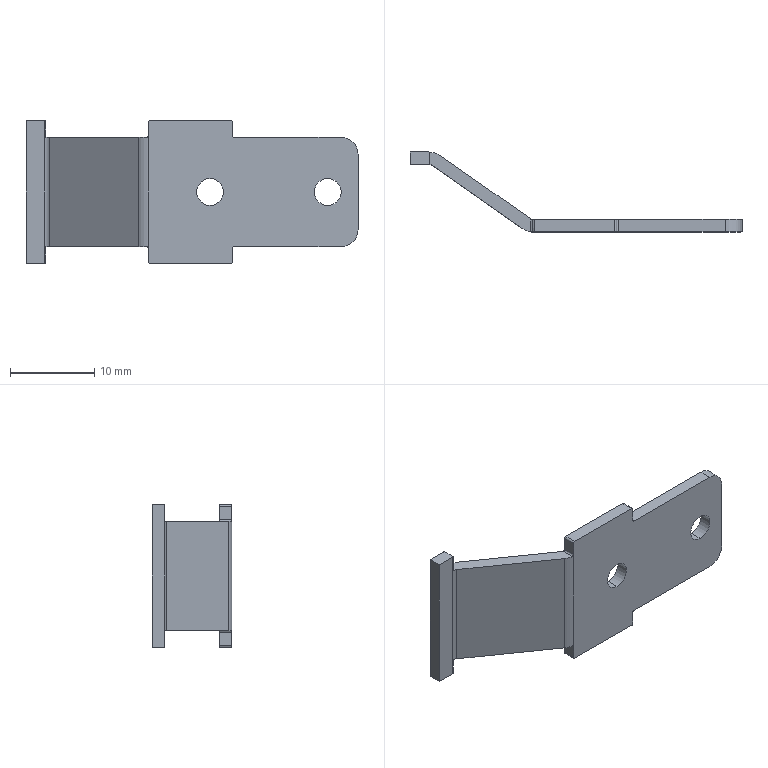Part | SolidWorks | features BaseBody 1 | 1 solid | 40 faces | box 39.5 x 9.5 x 17 mm | volume 865.542 mm3 | plane 22 | cylinder 18 | commonest cylinder face diameters 0.4 x8 3.2 x4 4 x3 1 x1 2 x1 6 x1
STEP:
#1=CARTESIAN_POINT('',(37.,-3.1,1.6));
#2=VERTEX_POINT('',#1);
#3=CARTESIAN_POINT('',(37.,-3.1,-1.6));
#4=VERTEX_POINT('',#3);
#5=CARTESIAN_POINT('',(37.,-3.1,0.));
#6=DIRECTION('',(0.,-1.,0.));
#7=DIRECTION('',(0.,0.,1.));
#8=AXIS2_PLACEMENT_3D('',#5,#6,#7);
#9=CIRCLE('',#8,1.6);
#10=EDGE_CURVE('',#2,#4,#9,.T.);
#11=ORIENTED_EDGE('',*,*,#10,.T.);
#12=CARTESIAN_POINT('',(37.,-1.6,-1.6));
#13=VERTEX_POINT('',#12);
#14=CARTESIAN_POINT('',(37.,20.,-1.6));
#15=DIRECTION('',(0.,1.,0.));
#16=VECTOR('',#15,1000.);
#17=LINE('',#14,#16);
#18=EDGE_CURVE('',#4,#13,#17,.T.);
#19=ORIENTED_EDGE('',*,*,#18,.T.);
#20=CARTESIAN_POINT('',(37.,-1.6,1.6));
#21=VERTEX_POINT('',#20);
#22=CARTESIAN_POINT('',(37.,-1.6,0.));
#23=DIRECTION('',(0.,-1.,0.));
#24=DIRECTION('',(0.,0.,1.));
#25=AXIS2_PLACEMENT_3D('',#22,#23,#24);
#26=CIRCLE('',#25,1.6);
#27=EDGE_CURVE('',#21,#13,#26,.T.);
#28=ORIENTED_EDGE('',*,*,#27,.F.);
#29=CARTESIAN_POINT('',(37.,20.,1.6));
#30=DIRECTION('',(0.,1.,0.));
#31=VECTOR('',#30,1000.);
#32=LINE('',#29,#31);
#33=EDGE_CURVE('',#2,#21,#32,.T.);
#34=ORIENTED_EDGE('',*,*,#33,.F.);
#35=EDGE_LOOP('',(#11,#19,#28,#34));
#36=FACE_OUTER_BOUND('',#35,.T.);
#37=CARTESIAN_POINT('',(37.,20.,0.));
#38=DIRECTION('',(0.,1.,0.));
#39=DIRECTION('',(0.,0.,1.));
#40=AXIS2_PLACEMENT_3D('',#37,#38,#39);
#41=CYLINDRICAL_SURFACE('',#40,1.6);
#42=ADVANCED_FACE('',(#36),#41,.F.);
#43=CARTESIAN_POINT('',(51.,-3.1,1.6));
#44=VERTEX_POINT('',#43);
#45=CARTESIAN_POINT('',(51.,-3.1,-1.6));
#46=VERTEX_POINT('',#45);
#47=CARTESIAN_POINT('',(51.,-3.1,0.));
#48=DIRECTION('',(0.,-1.,0.));
#49=DIRECTION('',(0.,0.,1.));
#50=AXIS2_PLACEMENT_3D('',#47,#48,#49);
#51=CIRCLE('',#50,1.6);
#52=EDGE_CURVE('',#44,#46,#51,.T.);
#53=ORIENTED_EDGE('',*,*,#52,.T.);
#54=CARTESIAN_POINT('',(51.,-1.6,-1.6));
#55=VERTEX_POINT('',#54);
#56=CARTESIAN_POINT('',(51.,20.,-1.6));
#57=DIRECTION('',(0.,1.,0.));
#58=VECTOR('',#57,1000.);
#59=LINE('',#56,#58);
#60=EDGE_CURVE('',#46,#55,#59,.T.);
#61=ORIENTED_EDGE('',*,*,#60,.T.);
#62=CARTESIAN_POINT('',(51.,-1.6,1.6));
#63=VERTEX_POINT('',#62);
#64=CARTESIAN_POINT('',(51.,-1.6,0.));
#65=DIRECTION('',(0.,-1.,0.));
#66=DIRECTION('',(0.,0.,1.));
#67=AXIS2_PLACEMENT_3D('',#64,#65,#66);
#68=CIRCLE('',#67,1.6);
#69=EDGE_CURVE('',#63,#55,#68,.T.);
#70=ORIENTED_EDGE('',*,*,#69,.F.);
#71=CARTESIAN_POINT('',(51.,20.,1.6));
#72=DIRECTION('',(0.,1.,0.));
#73=VECTOR('',#72,1000.);
#74=LINE('',#71,#73);
#75=EDGE_CURVE('',#44,#63,#74,.T.);
#76=ORIENTED_EDGE('',*,*,#75,.F.);
#77=EDGE_LOOP('',(#53,#61,#70,#76));
#78=FACE_OUTER_BOUND('',#77,.T.);
#79=CARTESIAN_POINT('',(51.,20.,0.));
#80=DIRECTION('',(0.,1.,0.));
#81=DIRECTION('',(0.,0.,1.));
#82=AXIS2_PLACEMENT_3D('',#79,#80,#81);
#83=CYLINDRICAL_SURFACE('',#82,1.6);
#84=ADVANCED_FACE('',(#78),#83,.F.);
#85=CARTESIAN_POINT('',(17.155,6.4,-8.5));
#86=VERTEX_POINT('',#85);
#87=CARTESIAN_POINT('',(15.1,6.4,-8.5));
#88=VERTEX_POINT('',#87);
#89=CARTESIAN_POINT('',(17.469,6.4,-8.5));
#90=DIRECTION('',(-1.,0.,0.));
#91=VECTOR('',#90,1000.);
#92=LINE('',#89,#91);
#93=EDGE_CURVE('',#86,#88,#92,.T.);
#94=ORIENTED_EDGE('',*,*,#93,.T.);
#95=CARTESIAN_POINT('',(15.1,6.4,8.5));
#96=VERTEX_POINT('',#95);
#97=CARTESIAN_POINT('',(15.1,6.4,20.));
#98=DIRECTION('',(0.,0.,1.));
#99=VECTOR('',#98,1000.);
#100=LINE('',#97,#99);
#101=EDGE_CURVE('',#88,#96,#100,.T.);
#102=ORIENTED_EDGE('',*,*,#101,.T.);
#103=CARTESIAN_POINT('',(17.155,6.4,8.5));
#104=VERTEX_POINT('',#103);
#105=CARTESIAN_POINT('',(15.1,6.4,8.5));
#106=DIRECTION('',(1.,0.,0.));
#107=VECTOR('',#106,1000.);
#108=LINE('',#105,#107);
#109=EDGE_CURVE('',#96,#104,#108,.T.);
#110=ORIENTED_EDGE('',*,*,#109,.T.);
#111=CARTESIAN_POINT('',(17.155,6.4,20.));
#112=DIRECTION('',(0.,0.,1.));
#113=VECTOR('',#112,1000.);
#114=LINE('',#111,#113);
#115=EDGE_CURVE('',#86,#104,#114,.T.);
#116=ORIENTED_EDGE('',*,*,#115,.F.);
#117=EDGE_LOOP('',(#94,#102,#110,#116));
#118=FACE_OUTER_BOUND('',#117,.T.);
#119=CARTESIAN_POINT('',(17.155,6.4,20.));
#120=DIRECTION('',(0.,-1.,0.));
#121=DIRECTION('',(0.,0.,-1.));
#122=AXIS2_PLACEMENT_3D('',#119,#120,#121);
#123=PLANE('',#122);
#124=ADVANCED_FACE('',(#118),#123,.F.);
#125=CARTESIAN_POINT('',(17.469,6.383,8.5));
#126=VERTEX_POINT('',#125);
#127=CARTESIAN_POINT('',(17.469,4.887,8.5));
#128=VERTEX_POINT('',#127);
#129=CARTESIAN_POINT('',(17.469,20.,8.5));
#130=DIRECTION('',(0.,-1.,0.));
#131=VECTOR('',#130,1000.);
#132=LINE('',#129,#131);
#133=EDGE_CURVE('',#126,#128,#132,.T.);
#134=ORIENTED_EDGE('',*,*,#133,.F.);
#135=CARTESIAN_POINT('',(17.155,3.4,8.5));
#136=DIRECTION('',(0.,0.,-1.));
#137=DIRECTION('',(1.,0.,0.));
#138=AXIS2_PLACEMENT_3D('',#135,#136,#137);
#139=CIRCLE('',#138,3.);
#140=EDGE_CURVE('',#104,#126,#139,.T.);
#141=ORIENTED_EDGE('',*,*,#140,.F.);
#142=ORIENTED_EDGE('',*,*,#109,.F.);
#143=CARTESIAN_POINT('',(15.1,4.9,8.5));
#144=VERTEX_POINT('',#143);
#145=CARTESIAN_POINT('',(15.1,6.4,8.5));
#146=DIRECTION('',(0.,-1.,0.));
#147=VECTOR('',#146,1000.);
#148=LINE('',#145,#147);
#149=EDGE_CURVE('',#96,#144,#148,.T.);
#150=ORIENTED_EDGE('',*,*,#149,.T.);
#151=CARTESIAN_POINT('',(17.311,4.9,8.5));
#152=VERTEX_POINT('',#151);
#153=CARTESIAN_POINT('',(15.1,4.9,8.5));
#154=DIRECTION('',(1.,0.,0.));
#155=VECTOR('',#154,1000.);
#156=LINE('',#153,#155);
#157=EDGE_CURVE('',#144,#152,#156,.T.);
#158=ORIENTED_EDGE('',*,*,#157,.T.);
#159=CARTESIAN_POINT('',(17.311,3.9,8.5));
#160=DIRECTION('',(0.,0.,1.));
#161=DIRECTION('',(1.,0.,0.));
#162=AXIS2_PLACEMENT_3D('',#159,#160,#161);
#163=CIRCLE('',#162,1.);
#164=EDGE_CURVE('',#128,#152,#163,.T.);
#165=ORIENTED_EDGE('',*,*,#164,.F.);
#166=EDGE_LOOP('',(#134,#141,#142,#150,#158,#165));
#167=FACE_OUTER_BOUND('',#166,.T.);
#168=CARTESIAN_POINT('',(15.1,20.,8.5));
#169=DIRECTION('',(0.,0.,-1.));
#170=DIRECTION('',(0.,-1.,0.));
#171=AXIS2_PLACEMENT_3D('',#168,#169,#170);
#172=PLANE('',#171);
#173=ADVANCED_FACE('',(#167),#172,.F.);
#174=ORIENTED_EDGE('',*,*,#93,.F.);
#175=CARTESIAN_POINT('',(17.469,6.383,-8.5));
#176=VERTEX_POINT('',#175);
#177=CARTESIAN_POINT('',(17.155,3.4,-8.5));
#178=DIRECTION('',(0.,0.,1.));
#179=DIRECTION('',(1.,0.,0.));
#180=AXIS2_PLACEMENT_3D('',#177,#178,#179);
#181=CIRCLE('',#180,3.);
#182=EDGE_CURVE('',#176,#86,#181,.T.);
#183=ORIENTED_EDGE('',*,*,#182,.F.);
#184=CARTESIAN_POINT('',(17.469,4.887,-8.5));
#185=VERTEX_POINT('',#184);
#186=CARTESIAN_POINT('',(17.469,20.,-8.5));
#187=DIRECTION('',(0.,1.,0.));
#188=VECTOR('',#187,1000.);
#189=LINE('',#186,#188);
#190=EDGE_CURVE('',#185,#176,#189,.T.);
#191=ORIENTED_EDGE('',*,*,#190,.F.);
#192=CARTESIAN_POINT('',(17.311,4.9,-8.5));
#193=VERTEX_POINT('',#192);
#194=CARTESIAN_POINT('',(17.311,3.9,-8.5));
#195=DIRECTION('',(0.,0.,-1.));
#196=DIRECTION('',(1.,0.,0.));
#197=AXIS2_PLACEMENT_3D('',#194,#195,#196);
#198=CIRCLE('',#197,1.);
#199=EDGE_CURVE('',#193,#185,#198,.T.);
#200=ORIENTED_EDGE('',*,*,#199,.F.);
#201=CARTESIAN_POINT('',(15.1,4.9,-8.5));
#202=VERTEX_POINT('',#201);
#203=CARTESIAN_POINT('',(15.1,4.9,-8.5));
#204=DIRECTION('',(-1.,0.,0.));
#205=VECTOR('',#204,1000.);
#206=LINE('',#203,#205);
#207=EDGE_CURVE('',#193,#202,#206,.T.);
#208=ORIENTED_EDGE('',*,*,#207,.T.);
#209=CARTESIAN_POINT('',(15.1,6.4,-8.5));
#210=DIRECTION('',(0.,1.,0.));
#211=VECTOR('',#210,1000.);
#212=LINE('',#209,#211);
#213=EDGE_CURVE('',#202,#88,#212,.T.);
#214=ORIENTED_EDGE('',*,*,#213,.T.);
#215=EDGE_LOOP('',(#174,#183,#191,#200,#208,#214));
#216=FACE_OUTER_BOUND('',#215,.T.);
#217=CARTESIAN_POINT('',(17.469,20.,-8.5));
#218=DIRECTION('',(0.,0.,1.));
#219=DIRECTION('',(1.,0.,0.));
#220=AXIS2_PLACEMENT_3D('',#217,#218,#219);
#221=PLANE('',#220);
#222=ADVANCED_FACE('',(#216),#221,.F.);
#223=ORIENTED_EDGE('',*,*,#213,.F.);
#224=CARTESIAN_POINT('',(15.1,4.9,20.));
#225=DIRECTION('',(0.,0.,1.));
#226=VECTOR('',#225,1000.);
#227=LINE('',#224,#226);
#228=EDGE_CURVE('',#202,#144,#227,.T.);
#229=ORIENTED_EDGE('',*,*,#228,.T.);
#230=ORIENTED_EDGE('',*,*,#149,.F.);
#231=ORIENTED_EDGE('',*,*,#101,.F.);
#232=EDGE_LOOP('',(#223,#229,#230,#231));
#233=FACE_OUTER_BOUND('',#232,.T.);
#234=CARTESIAN_POINT('',(15.1,6.4,20.));
#235=DIRECTION('',(1.,0.,0.));
#236=DIRECTION('',(0.,1.,0.));
#237=AXIS2_PLACEMENT_3D('',#234,#235,#236);
#238=PLANE('',#237);
#239=ADVANCED_FACE('',(#233),#238,.F.);
#240=CARTESIAN_POINT('',(18.875,5.857,6.5));
#241=VERTEX_POINT('',#240);
#242=CARTESIAN_POINT('',(18.875,5.857,-6.5));
#243=VERTEX_POINT('',#242);
#244=CARTESIAN_POINT('',(18.875,5.857,20.));
#245=DIRECTION('',(0.,0.,-1.));
#246=VECTOR('',#245,1000.);
#247=LINE('',#244,#246);
#248=EDGE_CURVE('',#241,#243,#247,.T.);
#249=ORIENTED_EDGE('',*,*,#248,.T.);
#250=CARTESIAN_POINT('',(17.469,6.383,-6.5));
#251=VERTEX_POINT('',#250);
#252=CARTESIAN_POINT('',(17.155,3.4,-6.5));
#253=DIRECTION('',(0.,0.,1.));
#254=DIRECTION('',(1.,0.,0.));
#255=AXIS2_PLACEMENT_3D('',#252,#253,#254);
#256=CIRCLE('',#255,3.);
#257=EDGE_CURVE('',#243,#251,#256,.T.);
#258=ORIENTED_EDGE('',*,*,#257,.T.);
#259=CARTESIAN_POINT('',(17.469,6.383,-6.5));
#260=DIRECTION('',(0.,0.,-1.));
#261=VECTOR('',#260,1000.);
#262=LINE('',#259,#261);
#263=EDGE_CURVE('',#251,#176,#262,.T.);
#264=ORIENTED_EDGE('',*,*,#263,.T.);
#265=ORIENTED_EDGE('',*,*,#182,.T.);
#266=ORIENTED_EDGE('',*,*,#115,.T.);
#267=ORIENTED_EDGE('',*,*,#140,.T.);
#268=CARTESIAN_POINT('',(17.469,6.383,6.5));
#269=VERTEX_POINT('',#268);
#270=CARTESIAN_POINT('',(17.469,6.383,8.5));
#271=DIRECTION('',(0.,0.,-1.));
#272=VECTOR('',#271,1000.);
#273=LINE('',#270,#272);
#274=EDGE_CURVE('',#126,#269,#273,.T.);
#275=ORIENTED_EDGE('',*,*,#274,.T.);
#276=CARTESIAN_POINT('',(17.155,3.4,6.5));
#277=DIRECTION('',(0.,0.,-1.));
#278=DIRECTION('',(1.,0.,0.));
#279=AXIS2_PLACEMENT_3D('',#276,#277,#278);
#280=CIRCLE('',#279,3.);
#281=EDGE_CURVE('',#269,#241,#280,.T.);
#282=ORIENTED_EDGE('',*,*,#281,.T.);
#283=EDGE_LOOP('',(#249,#258,#264,#265,#266,#267,#275,#282));
#284=FACE_OUTER_BOUND('',#283,.T.);
#285=CARTESIAN_POINT('',(17.155,3.4,20.));
#286=DIRECTION('',(0.,0.,1.));
#287=DIRECTION('',(1.,0.,0.));
#288=AXIS2_PLACEMENT_3D('',#285,#286,#287);
#289=CYLINDRICAL_SURFACE('',#288,3.);
#290=ADVANCED_FACE('',(#284),#289,.T.);
#291=ORIENTED_EDGE('',*,*,#207,.F.);
#292=CARTESIAN_POINT('',(17.311,4.9,20.));
#293=DIRECTION('',(0.,0.,1.));
#294=VECTOR('',#293,1000.);
#295=LINE('',#292,#294);
#296=EDGE_CURVE('',#193,#152,#295,.T.);
#297=ORIENTED_EDGE('',*,*,#296,.T.);
#298=ORIENTED_EDGE('',*,*,#157,.F.);
#299=ORIENTED_EDGE('',*,*,#228,.F.);
#300=EDGE_LOOP('',(#291,#297,#298,#299));
#301=FACE_OUTER_BOUND('',#300,.T.);
#302=CARTESIAN_POINT('',(15.1,4.9,20.));
#303=DIRECTION('',(0.,1.,0.));
#304=DIRECTION('',(1.,0.,0.));
#305=AXIS2_PLACEMENT_3D('',#302,#303,#304);
#306=PLANE('',#305);
#307=ADVANCED_FACE('',(#301),#306,.F.);
#308=CARTESIAN_POINT('',(17.469,4.887,6.5));
#309=VERTEX_POINT('',#308);
#310=CARTESIAN_POINT('',(17.469,20.,6.5));
#311=DIRECTION('',(0.,1.,0.));
#312=VECTOR('',#311,1000.);
#313=LINE('',#310,#312);
#314=EDGE_CURVE('',#309,#269,#313,.T.);
#315=ORIENTED_EDGE('',*,*,#314,.T.);
#316=ORIENTED_EDGE('',*,*,#274,.F.);
#317=ORIENTED_EDGE('',*,*,#133,.T.);
#318=CARTESIAN_POINT('',(17.469,4.887,20.));
#319=DIRECTION('',(0.,0.,-1.));
#320=VECTOR('',#319,1000.);
#321=LINE('',#318,#320);
#322=EDGE_CURVE('',#128,#309,#321,.T.);
#323=ORIENTED_EDGE('',*,*,#322,.T.);
#324=EDGE_LOOP('',(#315,#316,#317,#323));
#325=FACE_OUTER_BOUND('',#324,.T.);
#326=CARTESIAN_POINT('',(17.469,20.,8.5));
#327=DIRECTION('',(-1.,0.,0.));
#328=DIRECTION('',(0.,0.,1.));
#329=AXIS2_PLACEMENT_3D('',#326,#327,#328);
#330=PLANE('',#329);
#331=ADVANCED_FACE('',(#325),#330,.F.);
#332=ORIENTED_EDGE('',*,*,#190,.T.);
#333=ORIENTED_EDGE('',*,*,#263,.F.);
#334=CARTESIAN_POINT('',(17.469,4.887,-6.5));
#335=VERTEX_POINT('',#334);
#336=CARTESIAN_POINT('',(17.469,20.,-6.5));
#337=DIRECTION('',(0.,-1.,0.));
#338=VECTOR('',#337,1000.);
#339=LINE('',#336,#338);
#340=EDGE_CURVE('',#251,#335,#339,.T.);
#341=ORIENTED_EDGE('',*,*,#340,.T.);
#342=CARTESIAN_POINT('',(17.469,4.887,20.));
#343=DIRECTION('',(0.,0.,-1.));
#344=VECTOR('',#343,1000.);
#345=LINE('',#342,#344);
#346=EDGE_CURVE('',#335,#185,#345,.T.);
#347=ORIENTED_EDGE('',*,*,#346,.T.);
#348=EDGE_LOOP('',(#332,#333,#341,#347));
#349=FACE_OUTER_BOUND('',#348,.T.);
#350=CARTESIAN_POINT('',(17.469,20.,-6.5));
#351=DIRECTION('',(-1.,0.,0.));
#352=DIRECTION('',(0.,0.,1.));
#353=AXIS2_PLACEMENT_3D('',#350,#351,#352);
#354=PLANE('',#353);
#355=ADVANCED_FACE('',(#349),#354,.F.);
#356=CARTESIAN_POINT('',(29.397,-1.51,-6.5));
#357=VERTEX_POINT('',#356);
#358=CARTESIAN_POINT('',(29.397,-1.51,-6.5));
#359=DIRECTION('',(-0.8192,0.5736,0.));
#360=VECTOR('',#359,1000.);
#361=LINE('',#358,#360);
#362=EDGE_CURVE('',#357,#243,#361,.T.);
#363=ORIENTED_EDGE('',*,*,#362,.T.);
#364=ORIENTED_EDGE('',*,*,#248,.F.);
#365=CARTESIAN_POINT('',(29.397,-1.51,6.5));
#366=VERTEX_POINT('',#365);
#367=CARTESIAN_POINT('',(18.875,5.857,6.5));
#368=DIRECTION('',(0.8192,-0.5736,0.));
#369=VECTOR('',#368,1000.);
#370=LINE('',#367,#369);
#371=EDGE_CURVE('',#241,#366,#370,.T.);
#372=ORIENTED_EDGE('',*,*,#371,.T.);
#373=CARTESIAN_POINT('',(29.397,-1.51,20.));
#374=DIRECTION('',(0.,0.,-1.));
#375=VECTOR('',#374,1000.);
#376=LINE('',#373,#375);
#377=EDGE_CURVE('',#366,#357,#376,.T.);
#378=ORIENTED_EDGE('',*,*,#377,.T.);
#379=EDGE_LOOP('',(#363,#364,#372,#378));
#380=FACE_OUTER_BOUND('',#379,.T.);
#381=CARTESIAN_POINT('',(29.397,-1.51,20.));
#382=DIRECTION('',(-0.5736,-0.8192,0.));
#383=DIRECTION('',(-0.8192,0.5736,0.));
#384=AXIS2_PLACEMENT_3D('',#381,#382,#383);
#385=PLANE('',#384);
#386=ADVANCED_FACE('',(#380),#385,.F.);
#387=CARTESIAN_POINT('',(17.885,4.719,6.5));
#388=VERTEX_POINT('',#387);
#389=CARTESIAN_POINT('',(28.535,-2.738,6.5));
#390=VERTEX_POINT('',#389);
#391=CARTESIAN_POINT('',(17.885,4.719,6.5));
#392=DIRECTION('',(0.8192,-0.5736,0.));
#393=VECTOR('',#392,1000.);
#394=LINE('',#391,#393);
#395=EDGE_CURVE('',#388,#390,#394,.T.);
#396=ORIENTED_EDGE('',*,*,#395,.T.);
#397=CARTESIAN_POINT('',(29.483,-3.09,6.5));
#398=VERTEX_POINT('',#397);
#399=CARTESIAN_POINT('',(29.683,-1.1,6.5));
#400=DIRECTION('',(0.,0.,-1.));
#401=DIRECTION('',(1.,0.,0.));
#402=AXIS2_PLACEMENT_3D('',#399,#400,#401);
#403=CIRCLE('',#402,2.);
#404=EDGE_CURVE('',#398,#390,#403,.T.);
#405=ORIENTED_EDGE('',*,*,#404,.F.);
#406=CARTESIAN_POINT('',(29.483,-1.558,6.5));
#407=VERTEX_POINT('',#406);
#408=CARTESIAN_POINT('',(29.483,20.,6.5));
#409=DIRECTION('',(0.,-1.,0.));
#410=VECTOR('',#409,1000.);
#411=LINE('',#408,#410);
#412=EDGE_CURVE('',#407,#398,#411,.T.);
#413=ORIENTED_EDGE('',*,*,#412,.F.);
#414=CARTESIAN_POINT('',(29.684,-1.1,6.5));
#415=DIRECTION('',(0.,0.,-1.));
#416=DIRECTION('',(1.,0.,0.));
#417=AXIS2_PLACEMENT_3D('',#414,#415,#416);
#418=CIRCLE('',#417,0.5);
#419=EDGE_CURVE('',#407,#366,#418,.T.);
#420=ORIENTED_EDGE('',*,*,#419,.T.);
#421=ORIENTED_EDGE('',*,*,#371,.F.);
#422=ORIENTED_EDGE('',*,*,#281,.F.);
#423=ORIENTED_EDGE('',*,*,#314,.F.);
#424=CARTESIAN_POINT('',(17.311,3.9,6.5));
#425=DIRECTION('',(0.,0.,-1.));
#426=DIRECTION('',(1.,0.,0.));
#427=AXIS2_PLACEMENT_3D('',#424,#425,#426);
#428=CIRCLE('',#427,1.);
#429=EDGE_CURVE('',#309,#388,#428,.T.);
#430=ORIENTED_EDGE('',*,*,#429,.T.);
#431=EDGE_LOOP('',(#396,#405,#413,#420,#421,#422,#423,#430));
#432=FACE_OUTER_BOUND('',#431,.T.);
#433=CARTESIAN_POINT('',(17.469,20.,6.5));
#434=DIRECTION('',(0.,0.,-1.));
#435=DIRECTION('',(0.,-1.,0.));
#436=AXIS2_PLACEMENT_3D('',#433,#434,#435);
#437=PLANE('',#436);
#438=ADVANCED_FACE('',(#432),#437,.F.);
#439=ORIENTED_EDGE('',*,*,#340,.F.);
#440=ORIENTED_EDGE('',*,*,#257,.F.);
#441=ORIENTED_EDGE('',*,*,#362,.F.);
#442=CARTESIAN_POINT('',(29.483,-1.558,-6.5));
#443=VERTEX_POINT('',#442);
#444=CARTESIAN_POINT('',(29.684,-1.1,-6.5));
#445=DIRECTION('',(0.,0.,1.));
#446=DIRECTION('',(1.,0.,0.));
#447=AXIS2_PLACEMENT_3D('',#444,#445,#446);
#448=CIRCLE('',#447,0.5);
#449=EDGE_CURVE('',#357,#443,#448,.T.);
#450=ORIENTED_EDGE('',*,*,#449,.T.);
#451=CARTESIAN_POINT('',(29.483,-3.09,-6.5));
#452=VERTEX_POINT('',#451);
#453=CARTESIAN_POINT('',(29.483,20.,-6.5));
#454=DIRECTION('',(0.,1.,0.));
#455=VECTOR('',#454,1000.);
#456=LINE('',#453,#455);
#457=EDGE_CURVE('',#452,#443,#456,.T.);
#458=ORIENTED_EDGE('',*,*,#457,.F.);
#459=CARTESIAN_POINT('',(28.535,-2.738,-6.5));
#460=VERTEX_POINT('',#459);
#461=CARTESIAN_POINT('',(29.683,-1.1,-6.5));
#462=DIRECTION('',(0.,0.,1.));
#463=DIRECTION('',(1.,0.,0.));
#464=AXIS2_PLACEMENT_3D('',#461,#462,#463);
#465=CIRCLE('',#464,2.);
#466=EDGE_CURVE('',#460,#452,#465,.T.);
#467=ORIENTED_EDGE('',*,*,#466,.F.);
#468=CARTESIAN_POINT('',(17.885,4.719,-6.5));
#469=VERTEX_POINT('',#468);
#470=CARTESIAN_POINT('',(17.885,4.719,-6.5));
#471=DIRECTION('',(-0.8192,0.5736,0.));
#472=VECTOR('',#471,1000.);
#473=LINE('',#470,#472);
#474=EDGE_CURVE('',#460,#469,#473,.T.);
#475=ORIENTED_EDGE('',*,*,#474,.T.);
#476=CARTESIAN_POINT('',(17.311,3.9,-6.5));
#477=DIRECTION('',(0.,0.,1.));
#478=DIRECTION('',(1.,0.,0.));
#479=AXIS2_PLACEMENT_3D('',#476,#477,#478);
#480=CIRCLE('',#479,1.);
#481=EDGE_CURVE('',#469,#335,#480,.T.);
#482=ORIENTED_EDGE('',*,*,#481,.T.);
#483=EDGE_LOOP('',(#439,#440,#441,#450,#458,#467,#475,#482));
#484=FACE_OUTER_BOUND('',#483,.T.);
#485=CARTESIAN_POINT('',(29.483,20.,-6.5));
#486=DIRECTION('',(0.,0.,1.));
#487=DIRECTION('',(1.,0.,0.));
#488=AXIS2_PLACEMENT_3D('',#485,#486,#487);
#489=PLANE('',#488);
#490=ADVANCED_FACE('',(#484),#489,.F.);
#491=ORIENTED_EDGE('',*,*,#346,.F.);
#492=ORIENTED_EDGE('',*,*,#481,.F.);
#493=CARTESIAN_POINT('',(17.885,4.719,20.));
#494=DIRECTION('',(0.,0.,1.));
#495=VECTOR('',#494,1000.);
#496=LINE('',#493,#495);
#497=EDGE_CURVE('',#469,#388,#496,.T.);
#498=ORIENTED_EDGE('',*,*,#497,.T.);
#499=ORIENTED_EDGE('',*,*,#429,.F.);
#500=ORIENTED_EDGE('',*,*,#322,.F.);
#501=ORIENTED_EDGE('',*,*,#164,.T.);
#502=ORIENTED_EDGE('',*,*,#296,.F.);
#503=ORIENTED_EDGE('',*,*,#199,.T.);
#504=EDGE_LOOP('',(#491,#492,#498,#499,#500,#501,#502,#503));
#505=FACE_OUTER_BOUND('',#504,.T.);
#506=CARTESIAN_POINT('',(17.311,3.9,20.));
#507=DIRECTION('',(0.,0.,1.));
#508=DIRECTION('',(1.,0.,0.));
#509=AXIS2_PLACEMENT_3D('',#506,#507,#508);
#510=CYLINDRICAL_SURFACE('',#509,1.);
#511=ADVANCED_FACE('',(#505),#510,.F.);
#512=ORIENTED_EDGE('',*,*,#377,.F.);
#513=ORIENTED_EDGE('',*,*,#419,.F.);
#514=CARTESIAN_POINT('',(29.683,-1.6,6.7));
#515=VERTEX_POINT('',#514);
#516=CARTESIAN_POINT('',(29.483,-1.558,6.5));
#517=CARTESIAN_POINT('',(29.532,-1.58,6.5));
#518=CARTESIAN_POINT('',(29.585,-1.592,6.52));
#519=CARTESIAN_POINT('',(29.66,-1.601,6.594));
#520=CARTESIAN_POINT('',(29.683,-1.6,6.646));
#521=CARTESIAN_POINT('',(29.683,-1.6,6.7));
#522=B_SPLINE_CURVE_WITH_KNOTS('',3,(#516,#517,#518,#519,#520,#521),.UNSPECIFIED.,.F.,.F.,(4,2,4),(0.,0.000159,0.000318),.UNSPECIFIED.);
#523=EDGE_CURVE('',#407,#515,#522,.T.);
#524=ORIENTED_EDGE('',*,*,#523,.T.);
#525=CARTESIAN_POINT('',(29.683,-1.6,8.3));
#526=VERTEX_POINT('',#525);
#527=CARTESIAN_POINT('',(29.683,-1.6,20.));
#528=DIRECTION('',(0.,0.,-1.));
#529=VECTOR('',#528,1000.);
#530=LINE('',#527,#529);
#531=EDGE_CURVE('',#526,#515,#530,.T.);
#532=ORIENTED_EDGE('',*,*,#531,.F.);
#533=CARTESIAN_POINT('',(29.684,-1.6,8.316));
#534=VERTEX_POINT('',#533);
#535=CARTESIAN_POINT('',(29.883,-1.6,8.3));
#536=DIRECTION('',(0.,-1.,0.));
#537=DIRECTION('',(0.,0.,1.));
#538=AXIS2_PLACEMENT_3D('',#535,#536,#537);
#539=CIRCLE('',#538,0.2);
#540=EDGE_CURVE('',#534,#526,#539,.T.);
#541=ORIENTED_EDGE('',*,*,#540,.F.);
#542=CARTESIAN_POINT('',(29.684,-1.6,-8.316));
#543=VERTEX_POINT('',#542);
#544=CARTESIAN_POINT('',(29.684,-1.6,20.));
#545=DIRECTION('',(0.,0.,-1.));
#546=VECTOR('',#545,1000.);
#547=LINE('',#544,#546);
#548=EDGE_CURVE('',#534,#543,#547,.T.);
#549=ORIENTED_EDGE('',*,*,#548,.T.);
#550=CARTESIAN_POINT('',(29.683,-1.6,-8.3));
#551=VERTEX_POINT('',#550);
#552=CARTESIAN_POINT('',(29.883,-1.6,-8.3));
#553=DIRECTION('',(0.,-1.,0.));
#554=DIRECTION('',(0.,0.,1.));
#555=AXIS2_PLACEMENT_3D('',#552,#553,#554);
#556=CIRCLE('',#555,0.2);
#557=EDGE_CURVE('',#551,#543,#556,.T.);
#558=ORIENTED_EDGE('',*,*,#557,.F.);
#559=CARTESIAN_POINT('',(29.683,-1.6,-6.7));
#560=VERTEX_POINT('',#559);
#561=CARTESIAN_POINT('',(29.683,-1.6,20.));
#562=DIRECTION('',(0.,0.,-1.));
#563=VECTOR('',#562,1000.);
#564=LINE('',#561,#563);
#565=EDGE_CURVE('',#560,#551,#564,.T.);
#566=ORIENTED_EDGE('',*,*,#565,.F.);
#567=CARTESIAN_POINT('',(29.483,-1.558,-6.5));
#568=CARTESIAN_POINT('',(29.532,-1.58,-6.5));
#569=CARTESIAN_POINT('',(29.585,-1.592,-6.52));
#570=CARTESIAN_POINT('',(29.66,-1.601,-6.594));
#571=CARTESIAN_POINT('',(29.683,-1.6,-6.646));
#572=CARTESIAN_POINT('',(29.683,-1.6,-6.7));
#573=B_SPLINE_CURVE_WITH_KNOTS('',3,(#567,#568,#569,#570,#571,#572),.UNSPECIFIED.,.F.,.F.,(4,2,4),(0.,0.000159,0.000318),.UNSPECIFIED.);
#574=EDGE_CURVE('',#443,#560,#573,.T.);
#575=ORIENTED_EDGE('',*,*,#574,.F.);
#576=ORIENTED_EDGE('',*,*,#449,.F.);
#577=EDGE_LOOP('',(#512,#513,#524,#532,#541,#549,#558,#566,#575,#576));
#578=FACE_OUTER_BOUND('',#577,.T.);
#579=CARTESIAN_POINT('',(29.684,-1.1,20.));
#580=DIRECTION('',(0.,0.,1.));
#581=DIRECTION('',(1.,0.,0.));
#582=AXIS2_PLACEMENT_3D('',#579,#580,#581);
#583=CYLINDRICAL_SURFACE('',#582,0.5);
#584=ADVANCED_FACE('',(#578),#583,.F.);
#585=ORIENTED_EDGE('',*,*,#474,.F.);
#586=CARTESIAN_POINT('',(28.535,-2.738,20.));
#587=DIRECTION('',(0.,0.,-1.));
#588=VECTOR('',#587,1000.);
#589=LINE('',#586,#588);
#590=EDGE_CURVE('',#390,#460,#589,.T.);
#591=ORIENTED_EDGE('',*,*,#590,.F.);
#592=ORIENTED_EDGE('',*,*,#395,.F.);
#593=ORIENTED_EDGE('',*,*,#497,.F.);
#594=EDGE_LOOP('',(#585,#591,#592,#593));
#595=FACE_OUTER_BOUND('',#594,.T.);
#596=CARTESIAN_POINT('',(17.885,4.719,20.));
#597=DIRECTION('',(0.5736,0.8192,0.));
#598=DIRECTION('',(0.,0.,-1.));
#599=AXIS2_PLACEMENT_3D('',#596,#597,#598);
#600=PLANE('',#599);
#601=ADVANCED_FACE('',(#595),#600,.F.);
#602=CARTESIAN_POINT('',(29.683,-3.1,6.7));
#603=VERTEX_POINT('',#602);
#604=CARTESIAN_POINT('',(29.683,-3.1,6.687));
#605=VERTEX_POINT('',#604);
#606=CARTESIAN_POINT('',(29.483,-3.1,6.7));
#607=DIRECTION('',(0.,1.,0.));
#608=DIRECTION('',(0.,0.,1.));
#609=AXIS2_PLACEMENT_3D('',#606,#607,#608);
#610=CIRCLE('',#609,0.2);
#611=EDGE_CURVE('',#603,#605,#610,.T.);
#612=ORIENTED_EDGE('',*,*,#611,.F.);
#613=CARTESIAN_POINT('',(29.683,20.,6.7));
#614=DIRECTION('',(0.,1.,0.));
#615=VECTOR('',#614,1000.);
#616=LINE('',#613,#615);
#617=EDGE_CURVE('',#603,#515,#616,.T.);
#618=ORIENTED_EDGE('',*,*,#617,.T.);
#619=ORIENTED_EDGE('',*,*,#523,.F.);
#620=ORIENTED_EDGE('',*,*,#412,.T.);
#621=CARTESIAN_POINT('',(29.683,-3.1,6.687));
#622=CARTESIAN_POINT('',(29.679,-3.1,6.637));
#623=CARTESIAN_POINT('',(29.656,-3.1,6.588));
#624=CARTESIAN_POINT('',(29.583,-3.098,6.52));
#625=CARTESIAN_POINT('',(29.533,-3.095,6.5));
#626=CARTESIAN_POINT('',(29.483,-3.09,6.5));
#627=B_SPLINE_CURVE_WITH_KNOTS('',3,(#621,#622,#623,#624,#625,#626),.UNSPECIFIED.,.F.,.F.,(4,2,4),(0.,0.00015,0.0003),.UNSPECIFIED.);
#628=EDGE_CURVE('',#605,#398,#627,.T.);
#629=ORIENTED_EDGE('',*,*,#628,.F.);
#630=EDGE_LOOP('',(#612,#618,#619,#620,#629));
#631=FACE_OUTER_BOUND('',#630,.T.);
#632=CARTESIAN_POINT('',(29.483,20.,6.7));
#633=DIRECTION('',(0.,1.,0.));
#634=DIRECTION('',(0.,0.,1.));
#635=AXIS2_PLACEMENT_3D('',#632,#633,#634);
#636=CYLINDRICAL_SURFACE('',#635,0.2);
#637=ADVANCED_FACE('',(#631),#636,.F.);
#638=CARTESIAN_POINT('',(29.683,-3.1,8.3));
#639=VERTEX_POINT('',#638);
#640=CARTESIAN_POINT('',(29.683,20.,8.3));
#641=DIRECTION('',(0.,-1.,0.));
#642=VECTOR('',#641,1000.);
#643=LINE('',#640,#642);
#644=EDGE_CURVE('',#526,#639,#643,.T.);
#645=ORIENTED_EDGE('',*,*,#644,.T.);
#646=CARTESIAN_POINT('',(29.883,-3.1,8.5));
#647=VERTEX_POINT('',#646);
#648=CARTESIAN_POINT('',(29.883,-3.1,8.3));
#649=DIRECTION('',(0.,1.,0.));
#650=DIRECTION('',(0.,0.,1.));
#651=AXIS2_PLACEMENT_3D('',#648,#649,#650);
#652=CIRCLE('',#651,0.2);
#653=EDGE_CURVE('',#639,#647,#652,.T.);
#654=ORIENTED_EDGE('',*,*,#653,.T.);
#655=CARTESIAN_POINT('',(29.883,-1.6,8.5));
#656=VERTEX_POINT('',#655);
#657=CARTESIAN_POINT('',(29.883,20.,8.5));
#658=DIRECTION('',(0.,1.,0.));
#659=VECTOR('',#658,1000.);
#660=LINE('',#657,#659);
#661=EDGE_CURVE('',#647,#656,#660,.T.);
#662=ORIENTED_EDGE('',*,*,#661,.T.);
#663=CARTESIAN_POINT('',(29.883,-1.6,8.3));
#664=DIRECTION('',(0.,-1.,0.));
#665=DIRECTION('',(0.,0.,1.));
#666=AXIS2_PLACEMENT_3D('',#663,#664,#665);
#667=CIRCLE('',#666,0.2);
#668=EDGE_CURVE('',#656,#534,#667,.T.);
#669=ORIENTED_EDGE('',*,*,#668,.T.);
#670=ORIENTED_EDGE('',*,*,#540,.T.);
#671=EDGE_LOOP('',(#645,#654,#662,#669,#670));
#672=FACE_OUTER_BOUND('',#671,.T.);
#673=CARTESIAN_POINT('',(29.883,20.,8.3));
#674=DIRECTION('',(0.,1.,0.));
#675=DIRECTION('',(0.,0.,1.));
#676=AXIS2_PLACEMENT_3D('',#673,#674,#675);
#677=CYLINDRICAL_SURFACE('',#676,0.2);
#678=ADVANCED_FACE('',(#672),#677,.T.);
#679=CARTESIAN_POINT('',(39.483,-1.6,8.5));
#680=VERTEX_POINT('',#679);
#681=CARTESIAN_POINT('',(39.483,-3.1,8.5));
#682=VERTEX_POINT('',#681);
#683=CARTESIAN_POINT('',(39.483,20.,8.5));
#684=DIRECTION('',(0.,-1.,0.));
#685=VECTOR('',#684,1000.);
#686=LINE('',#683,#685);
#687=EDGE_CURVE('',#680,#682,#686,.T.);
#688=ORIENTED_EDGE('',*,*,#687,.T.);
#689=CARTESIAN_POINT('',(39.683,-3.1,8.3));
#690=VERTEX_POINT('',#689);
#691=CARTESIAN_POINT('',(39.483,-3.1,8.3));
#692=DIRECTION('',(0.,1.,0.));
#693=DIRECTION('',(0.,0.,1.));
#694=AXIS2_PLACEMENT_3D('',#691,#692,#693);
#695=CIRCLE('',#694,0.2);
#696=EDGE_CURVE('',#682,#690,#695,.T.);
#697=ORIENTED_EDGE('',*,*,#696,.T.);
#698=CARTESIAN_POINT('',(39.683,-1.6,8.3));
#699=VERTEX_POINT('',#698);
#700=CARTESIAN_POINT('',(39.683,20.,8.3));
#701=DIRECTION('',(0.,1.,0.));
#702=VECTOR('',#701,1000.);
#703=LINE('',#700,#702);
#704=EDGE_CURVE('',#690,#699,#703,.T.);
#705=ORIENTED_EDGE('',*,*,#704,.T.);
#706=CARTESIAN_POINT('',(39.483,-1.6,8.3));
#707=DIRECTION('',(0.,-1.,0.));
#708=DIRECTION('',(0.,0.,1.));
#709=AXIS2_PLACEMENT_3D('',#706,#707,#708);
#710=CIRCLE('',#709,0.2);
#711=EDGE_CURVE('',#699,#680,#710,.T.);
#712=ORIENTED_EDGE('',*,*,#711,.T.);
#713=EDGE_LOOP('',(#688,#697,#705,#712));
#714=FACE_OUTER_BOUND('',#713,.T.);
#715=CARTESIAN_POINT('',(39.483,20.,8.3));
#716=DIRECTION('',(0.,1.,0.));
#717=DIRECTION('',(0.,0.,1.));
#718=AXIS2_PLACEMENT_3D('',#715,#716,#717);
#719=CYLINDRICAL_SURFACE('',#718,0.2);
#720=ADVANCED_FACE('',(#714),#719,.T.);
#721=CARTESIAN_POINT('',(39.883,-3.1,6.5));
#722=VERTEX_POINT('',#721);
#723=CARTESIAN_POINT('',(39.883,-1.6,6.5));
#724=VERTEX_POINT('',#723);
#725=CARTESIAN_POINT('',(39.883,20.,6.5));
#726=DIRECTION('',(0.,1.,0.));
#727=VECTOR('',#726,1000.);
#728=LINE('',#725,#727);
#729=EDGE_CURVE('',#722,#724,#728,.T.);
#730=ORIENTED_EDGE('',*,*,#729,.T.);
#731=CARTESIAN_POINT('',(39.683,-1.6,6.7));
#732=VERTEX_POINT('',#731);
#733=CARTESIAN_POINT('',(39.883,-1.6,6.7));
#734=DIRECTION('',(0.,1.,0.));
#735=DIRECTION('',(0.,0.,1.));
#736=AXIS2_PLACEMENT_3D('',#733,#734,#735);
#737=CIRCLE('',#736,0.2);
#738=EDGE_CURVE('',#724,#732,#737,.T.);
#739=ORIENTED_EDGE('',*,*,#738,.T.);
#740=CARTESIAN_POINT('',(39.683,-3.1,6.7));
#741=VERTEX_POINT('',#740);
#742=CARTESIAN_POINT('',(39.683,20.,6.7));
#743=DIRECTION('',(0.,-1.,0.));
#744=VECTOR('',#743,1000.);
#745=LINE('',#742,#744);
#746=EDGE_CURVE('',#732,#741,#745,.T.);
#747=ORIENTED_EDGE('',*,*,#746,.T.);
#748=CARTESIAN_POINT('',(39.883,-3.1,6.7));
#749=DIRECTION('',(0.,1.,0.));
#750=DIRECTION('',(0.,0.,1.));
#751=AXIS2_PLACEMENT_3D('',#748,#749,#750);
#752=CIRCLE('',#751,0.2);
#753=EDGE_CURVE('',#722,#741,#752,.T.);
#754=ORIENTED_EDGE('',*,*,#753,.F.);
#755=EDGE_LOOP('',(#730,#739,#747,#754));
#756=FACE_OUTER_BOUND('',#755,.T.);
#757=CARTESIAN_POINT('',(39.883,20.,6.7));
#758=DIRECTION('',(0.,1.,0.));
#759=DIRECTION('',(0.,0.,1.));
#760=AXIS2_PLACEMENT_3D('',#757,#758,#759);
#761=CYLINDRICAL_SURFACE('',#760,0.2);
#762=ADVANCED_FACE('',(#756),#761,.F.);
#763=CARTESIAN_POINT('',(39.683,-3.1,-6.7));
#764=VERTEX_POINT('',#763);
#765=CARTESIAN_POINT('',(39.683,-1.6,-6.7));
#766=VERTEX_POINT('',#765);
#767=CARTESIAN_POINT('',(39.683,20.,-6.7));
#768=DIRECTION('',(0.,1.,0.));
#769=VECTOR('',#768,1000.);
#770=LINE('',#767,#769);
#771=EDGE_CURVE('',#764,#766,#770,.T.);
#772=ORIENTED_EDGE('',*,*,#771,.T.);
#773=CARTESIAN_POINT('',(39.883,-1.6,-6.5));
#774=VERTEX_POINT('',#773);
#775=CARTESIAN_POINT('',(39.883,-1.6,-6.7));
#776=DIRECTION('',(0.,1.,0.));
#777=DIRECTION('',(0.,0.,1.));
#778=AXIS2_PLACEMENT_3D('',#775,#776,#777);
#779=CIRCLE('',#778,0.2);
#780=EDGE_CURVE('',#766,#774,#779,.T.);
#781=ORIENTED_EDGE('',*,*,#780,.T.);
#782=CARTESIAN_POINT('',(39.883,-3.1,-6.5));
#783=VERTEX_POINT('',#782);
#784=CARTESIAN_POINT('',(39.883,20.,-6.5));
#785=DIRECTION('',(0.,-1.,0.));
#786=VECTOR('',#785,1000.);
#787=LINE('',#784,#786);
#788=EDGE_CURVE('',#774,#783,#787,.T.);
#789=ORIENTED_EDGE('',*,*,#788,.T.);
#790=CARTESIAN_POINT('',(39.883,-3.1,-6.7));
#791=DIRECTION('',(0.,1.,0.));
#792=DIRECTION('',(0.,0.,1.));
#793=AXIS2_PLACEMENT_3D('',#790,#791,#792);
#794=CIRCLE('',#793,0.2);
#795=EDGE_CURVE('',#764,#783,#794,.T.);
#796=ORIENTED_EDGE('',*,*,#795,.F.);
#797=EDGE_LOOP('',(#772,#781,#789,#796));
#798=FACE_OUTER_BOUND('',#797,.T.);
#799=CARTESIAN_POINT('',(39.883,20.,-6.7));
#800=DIRECTION('',(0.,1.,0.));
#801=DIRECTION('',(0.,0.,1.));
#802=AXIS2_PLACEMENT_3D('',#799,#800,#801);
#803=CYLINDRICAL_SURFACE('',#802,0.2);
#804=ADVANCED_FACE('',(#798),#803,.F.);
#805=CARTESIAN_POINT('',(39.683,-1.6,-8.3));
#806=VERTEX_POINT('',#805);
#807=CARTESIAN_POINT('',(39.683,-3.1,-8.3));
#808=VERTEX_POINT('',#807);
#809=CARTESIAN_POINT('',(39.683,20.,-8.3));
#810=DIRECTION('',(0.,-1.,0.));
#811=VECTOR('',#810,1000.);
#812=LINE('',#809,#811);
#813=EDGE_CURVE('',#806,#808,#812,.T.);
#814=ORIENTED_EDGE('',*,*,#813,.T.);
#815=CARTESIAN_POINT('',(39.483,-3.1,-8.5));
#816=VERTEX_POINT('',#815);
#817=CARTESIAN_POINT('',(39.483,-3.1,-8.3));
#818=DIRECTION('',(0.,1.,0.));
#819=DIRECTION('',(0.,0.,1.));
#820=AXIS2_PLACEMENT_3D('',#817,#818,#819);
#821=CIRCLE('',#820,0.2);
#822=EDGE_CURVE('',#808,#816,#821,.T.);
#823=ORIENTED_EDGE('',*,*,#822,.T.);
#824=CARTESIAN_POINT('',(39.483,-1.6,-8.5));
#825=VERTEX_POINT('',#824);
#826=CARTESIAN_POINT('',(39.483,20.,-8.5));
#827=DIRECTION('',(0.,1.,0.));
#828=VECTOR('',#827,1000.);
#829=LINE('',#826,#828);
#830=EDGE_CURVE('',#816,#825,#829,.T.);
#831=ORIENTED_EDGE('',*,*,#830,.T.);
#832=CARTESIAN_POINT('',(39.483,-1.6,-8.3));
#833=DIRECTION('',(0.,-1.,0.));
#834=DIRECTION('',(0.,0.,1.));
#835=AXIS2_PLACEMENT_3D('',#832,#833,#834);
#836=CIRCLE('',#835,0.2);
#837=EDGE_CURVE('',#825,#806,#836,.T.);
#838=ORIENTED_EDGE('',*,*,#837,.T.);
#839=EDGE_LOOP('',(#814,#823,#831,#838));
#840=FACE_OUTER_BOUND('',#839,.T.);
#841=CARTESIAN_POINT('',(39.483,20.,-8.3));
#842=DIRECTION('',(0.,1.,0.));
#843=DIRECTION('',(0.,0.,1.));
#844=AXIS2_PLACEMENT_3D('',#841,#842,#843);
#845=CYLINDRICAL_SURFACE('',#844,0.2);
#846=ADVANCED_FACE('',(#840),#845,.T.);
#847=ORIENTED_EDGE('',*,*,#69,.T.);
#848=CARTESIAN_POINT('',(51.,-1.6,0.));
#849=DIRECTION('',(0.,-1.,0.));
#850=DIRECTION('',(0.,0.,1.));
#851=AXIS2_PLACEMENT_3D('',#848,#849,#850);
#852=CIRCLE('',#851,1.6);
#853=EDGE_CURVE('',#55,#63,#852,.T.);
#854=ORIENTED_EDGE('',*,*,#853,.T.);
#855=EDGE_LOOP('',(#847,#854));
#856=FACE_BOUND('',#855,.T.);
#857=ORIENTED_EDGE('',*,*,#27,.T.);
#858=CARTESIAN_POINT('',(37.,-1.6,0.));
#859=DIRECTION('',(0.,-1.,0.));
#860=DIRECTION('',(0.,0.,1.));
#861=AXIS2_PLACEMENT_3D('',#858,#859,#860);
#862=CIRCLE('',#861,1.6);
#863=EDGE_CURVE('',#13,#21,#862,.T.);
#864=ORIENTED_EDGE('',*,*,#863,.T.);
#865=EDGE_LOOP('',(#857,#864));
#866=FACE_BOUND('',#865,.T.);
#867=CARTESIAN_POINT('',(29.883,-1.6,-8.5));
#868=VERTEX_POINT('',#867);
#869=CARTESIAN_POINT('',(29.883,-1.6,-8.3));
#870=DIRECTION('',(0.,-1.,0.));
#871=DIRECTION('',(0.,0.,1.));
#872=AXIS2_PLACEMENT_3D('',#869,#870,#871);
#873=CIRCLE('',#872,0.2);
#874=EDGE_CURVE('',#543,#868,#873,.T.);
#875=ORIENTED_EDGE('',*,*,#874,.F.);
#876=ORIENTED_EDGE('',*,*,#548,.F.);
#877=ORIENTED_EDGE('',*,*,#668,.F.);
#878=CARTESIAN_POINT('',(29.883,-1.6,8.5));
#879=DIRECTION('',(1.,0.,0.));
#880=VECTOR('',#879,1000.);
#881=LINE('',#878,#880);
#882=EDGE_CURVE('',#656,#680,#881,.T.);
#883=ORIENTED_EDGE('',*,*,#882,.T.);
#884=ORIENTED_EDGE('',*,*,#711,.F.);
#885=CARTESIAN_POINT('',(39.683,-1.6,8.3));
#886=DIRECTION('',(0.,0.,-1.));
#887=VECTOR('',#886,1000.);
#888=LINE('',#885,#887);
#889=EDGE_CURVE('',#699,#732,#888,.T.);
#890=ORIENTED_EDGE('',*,*,#889,.T.);
#891=ORIENTED_EDGE('',*,*,#738,.F.);
#892=CARTESIAN_POINT('',(52.6,-1.6,6.5));
#893=VERTEX_POINT('',#892);
#894=CARTESIAN_POINT('',(39.883,-1.6,6.5));
#895=DIRECTION('',(1.,0.,0.));
#896=VECTOR('',#895,1000.);
#897=LINE('',#894,#896);
#898=EDGE_CURVE('',#724,#893,#897,.T.);
#899=ORIENTED_EDGE('',*,*,#898,.T.);
#900=CARTESIAN_POINT('',(54.6,-1.6,4.5));
#901=VERTEX_POINT('',#900);
#902=CARTESIAN_POINT('',(52.6,-1.6,4.5));
#903=DIRECTION('',(0.,-1.,0.));
#904=DIRECTION('',(0.,0.,1.));
#905=AXIS2_PLACEMENT_3D('',#902,#903,#904);
#906=CIRCLE('',#905,2.);
#907=EDGE_CURVE('',#901,#893,#906,.T.);
#908=ORIENTED_EDGE('',*,*,#907,.F.);
#909=CARTESIAN_POINT('',(54.6,-1.6,-4.5));
#910=VERTEX_POINT('',#909);
#911=CARTESIAN_POINT('',(54.6,-1.6,20.));
#912=DIRECTION('',(0.,0.,-1.));
#913=VECTOR('',#912,1000.);
#914=LINE('',#911,#913);
#915=EDGE_CURVE('',#901,#910,#914,.T.);
#916=ORIENTED_EDGE('',*,*,#915,.T.);
#917=CARTESIAN_POINT('',(52.6,-1.6,-6.5));
#918=VERTEX_POINT('',#917);
#919=CARTESIAN_POINT('',(52.6,-1.6,-4.5));
#920=DIRECTION('',(0.,-1.,0.));
#921=DIRECTION('',(0.,0.,1.));
#922=AXIS2_PLACEMENT_3D('',#919,#920,#921);
#923=CIRCLE('',#922,2.);
#924=EDGE_CURVE('',#918,#910,#923,.T.);
#925=ORIENTED_EDGE('',*,*,#924,.F.);
#926=CARTESIAN_POINT('',(52.6,-1.6,-6.5));
#927=DIRECTION('',(-1.,0.,0.));
#928=VECTOR('',#927,1000.);
#929=LINE('',#926,#928);
#930=EDGE_CURVE('',#918,#774,#929,.T.);
#931=ORIENTED_EDGE('',*,*,#930,.T.);
#932=ORIENTED_EDGE('',*,*,#780,.F.);
#933=CARTESIAN_POINT('',(39.683,-1.6,-6.7));
#934=DIRECTION('',(0.,0.,-1.));
#935=VECTOR('',#934,1000.);
#936=LINE('',#933,#935);
#937=EDGE_CURVE('',#766,#806,#936,.T.);
#938=ORIENTED_EDGE('',*,*,#937,.T.);
#939=ORIENTED_EDGE('',*,*,#837,.F.);
#940=CARTESIAN_POINT('',(39.483,-1.6,-8.5));
#941=DIRECTION('',(-1.,0.,0.));
#942=VECTOR('',#941,1000.);
#943=LINE('',#940,#942);
#944=EDGE_CURVE('',#825,#868,#943,.T.);
#945=ORIENTED_EDGE('',*,*,#944,.T.);
#946=EDGE_LOOP('',(#875,#876,#877,#883,#884,#890,#891,#899,#908,#916,#925,#931,#932,#938,#939,#945));
#947=FACE_OUTER_BOUND('',#946,.T.);
#948=CARTESIAN_POINT('',(54.6,-1.6,20.));
#949=DIRECTION('',(0.,-1.,0.));
#950=DIRECTION('',(0.,0.,-1.));
#951=AXIS2_PLACEMENT_3D('',#948,#949,#950);
#952=PLANE('',#951);
#953=ADVANCED_FACE('',(#856,#866,#947),#952,.F.);
#954=CARTESIAN_POINT('',(29.883,-3.1,-8.5));
#955=VERTEX_POINT('',#954);
#956=CARTESIAN_POINT('',(29.883,20.,-8.5));
#957=DIRECTION('',(0.,-1.,0.));
#958=VECTOR('',#957,1000.);
#959=LINE('',#956,#958);
#960=EDGE_CURVE('',#868,#955,#959,.T.);
#961=ORIENTED_EDGE('',*,*,#960,.T.);
#962=CARTESIAN_POINT('',(29.683,-3.1,-8.3));
#963=VERTEX_POINT('',#962);
#964=CARTESIAN_POINT('',(29.883,-3.1,-8.3));
#965=DIRECTION('',(0.,1.,0.));
#966=DIRECTION('',(0.,0.,1.));
#967=AXIS2_PLACEMENT_3D('',#964,#965,#966);
#968=CIRCLE('',#967,0.2);
#969=EDGE_CURVE('',#955,#963,#968,.T.);
#970=ORIENTED_EDGE('',*,*,#969,.T.);
#971=CARTESIAN_POINT('',(29.683,20.,-8.3));
#972=DIRECTION('',(0.,1.,0.));
#973=VECTOR('',#972,1000.);
#974=LINE('',#971,#973);
#975=EDGE_CURVE('',#963,#551,#974,.T.);
#976=ORIENTED_EDGE('',*,*,#975,.T.);
#977=ORIENTED_EDGE('',*,*,#557,.T.);
#978=ORIENTED_EDGE('',*,*,#874,.T.);
#979=EDGE_LOOP('',(#961,#970,#976,#977,#978));
#980=FACE_OUTER_BOUND('',#979,.T.);
#981=CARTESIAN_POINT('',(29.883,20.,-8.3));
#982=DIRECTION('',(0.,1.,0.));
#983=DIRECTION('',(0.,0.,1.));
#984=AXIS2_PLACEMENT_3D('',#981,#982,#983);
#985=CYLINDRICAL_SURFACE('',#984,0.2);
#986=ADVANCED_FACE('',(#980),#985,.T.);
#987=ORIENTED_EDGE('',*,*,#457,.T.);
#988=ORIENTED_EDGE('',*,*,#574,.T.);
#989=CARTESIAN_POINT('',(29.683,-3.1,-6.7));
#990=VERTEX_POINT('',#989);
#991=CARTESIAN_POINT('',(29.683,20.,-6.7));
#992=DIRECTION('',(0.,-1.,0.));
#993=VECTOR('',#992,1000.);
#994=LINE('',#991,#993);
#995=EDGE_CURVE('',#560,#990,#994,.T.);
#996=ORIENTED_EDGE('',*,*,#995,.T.);
#997=CARTESIAN_POINT('',(29.683,-3.1,-6.687));
#998=VERTEX_POINT('',#997);
#999=CARTESIAN_POINT('',(29.483,-3.1,-6.7));
#1000=DIRECTION('',(0.,1.,0.));
#1001=DIRECTION('',(0.,0.,1.));
#1002=AXIS2_PLACEMENT_3D('',#999,#1000,#1001);
#1003=CIRCLE('',#1002,0.2);
#1004=EDGE_CURVE('',#998,#990,#1003,.T.);
#1005=ORIENTED_EDGE('',*,*,#1004,.F.);
#1006=CARTESIAN_POINT('',(29.483,-3.09,-6.5));
#1007=CARTESIAN_POINT('',(29.533,-3.095,-6.5));
#1008=CARTESIAN_POINT('',(29.583,-3.098,-6.52));
#1009=CARTESIAN_POINT('',(29.656,-3.1,-6.588));
#1010=CARTESIAN_POINT('',(29.679,-3.1,-6.637));
#1011=CARTESIAN_POINT('',(29.683,-3.1,-6.687));
#1012=B_SPLINE_CURVE_WITH_KNOTS('',3,(#1006,#1007,#1008,#1009,#1010,#1011),.UNSPECIFIED.,.F.,.F.,(4,2,4),(0.,0.00015,0.0003),.UNSPECIFIED.);
#1013=EDGE_CURVE('',#452,#998,#1012,.T.);
#1014=ORIENTED_EDGE('',*,*,#1013,.F.);
#1015=EDGE_LOOP('',(#987,#988,#996,#1005,#1014));
#1016=FACE_OUTER_BOUND('',#1015,.T.);
#1017=CARTESIAN_POINT('',(29.483,20.,-6.7));
#1018=DIRECTION('',(0.,1.,0.));
#1019=DIRECTION('',(0.,0.,1.));
#1020=AXIS2_PLACEMENT_3D('',#1017,#1018,#1019);
#1021=CYLINDRICAL_SURFACE('',#1020,0.2);
#1022=ADVANCED_FACE('',(#1016),#1021,.F.);
#1023=ORIENTED_EDGE('',*,*,#628,.T.);
#1024=ORIENTED_EDGE('',*,*,#404,.T.);
#1025=ORIENTED_EDGE('',*,*,#590,.T.);
#1026=ORIENTED_EDGE('',*,*,#466,.T.);
#1027=ORIENTED_EDGE('',*,*,#1013,.T.);
#1028=CARTESIAN_POINT('',(29.683,-3.1,20.));
#1029=DIRECTION('',(0.,0.,1.));
#1030=VECTOR('',#1029,1000.);
#1031=LINE('',#1028,#1030);
#1032=EDGE_CURVE('',#998,#605,#1031,.T.);
#1033=ORIENTED_EDGE('',*,*,#1032,.T.);
#1034=EDGE_LOOP('',(#1023,#1024,#1025,#1026,#1027,#1033));
#1035=FACE_OUTER_BOUND('',#1034,.T.);
#1036=CARTESIAN_POINT('',(29.683,-1.1,20.));
#1037=DIRECTION('',(0.,0.,1.));
#1038=DIRECTION('',(1.,0.,0.));
#1039=AXIS2_PLACEMENT_3D('',#1036,#1037,#1038);
#1040=CYLINDRICAL_SURFACE('',#1039,2.);
#1041=ADVANCED_FACE('',(#1035),#1040,.T.);
#1042=ORIENTED_EDGE('',*,*,#531,.T.);
#1043=ORIENTED_EDGE('',*,*,#617,.F.);
#1044=CARTESIAN_POINT('',(29.683,-3.1,20.));
#1045=DIRECTION('',(0.,0.,1.));
#1046=VECTOR('',#1045,1000.);
#1047=LINE('',#1044,#1046);
#1048=EDGE_CURVE('',#603,#639,#1047,.T.);
#1049=ORIENTED_EDGE('',*,*,#1048,.T.);
#1050=ORIENTED_EDGE('',*,*,#644,.F.);
#1051=EDGE_LOOP('',(#1042,#1043,#1049,#1050));
#1052=FACE_OUTER_BOUND('',#1051,.T.);
#1053=CARTESIAN_POINT('',(29.683,20.,6.7));
#1054=DIRECTION('',(1.,0.,0.));
#1055=DIRECTION('',(0.,1.,0.));
#1056=AXIS2_PLACEMENT_3D('',#1053,#1054,#1055);
#1057=PLANE('',#1056);
#1058=ADVANCED_FACE('',(#1052),#1057,.F.);
#1059=ORIENTED_EDGE('',*,*,#882,.F.);
#1060=ORIENTED_EDGE('',*,*,#661,.F.);
#1061=CARTESIAN_POINT('',(29.683,-3.1,8.5));
#1062=DIRECTION('',(1.,0.,0.));
#1063=VECTOR('',#1062,1000.);
#1064=LINE('',#1061,#1063);
#1065=EDGE_CURVE('',#647,#682,#1064,.T.);
#1066=ORIENTED_EDGE('',*,*,#1065,.T.);
#1067=ORIENTED_EDGE('',*,*,#687,.F.);
#1068=EDGE_LOOP('',(#1059,#1060,#1066,#1067));
#1069=FACE_OUTER_BOUND('',#1068,.T.);
#1070=CARTESIAN_POINT('',(29.883,20.,8.5));
#1071=DIRECTION('',(0.,0.,-1.));
#1072=DIRECTION('',(0.,-1.,0.));
#1073=AXIS2_PLACEMENT_3D('',#1070,#1071,#1072);
#1074=PLANE('',#1073);
#1075=ADVANCED_FACE('',(#1069),#1074,.F.);
#1076=ORIENTED_EDGE('',*,*,#889,.F.);
#1077=ORIENTED_EDGE('',*,*,#704,.F.);
#1078=CARTESIAN_POINT('',(39.683,-3.1,20.));
#1079=DIRECTION('',(0.,0.,-1.));
#1080=VECTOR('',#1079,1000.);
#1081=LINE('',#1078,#1080);
#1082=EDGE_CURVE('',#690,#741,#1081,.T.);
#1083=ORIENTED_EDGE('',*,*,#1082,.T.);
#1084=ORIENTED_EDGE('',*,*,#746,.F.);
#1085=EDGE_LOOP('',(#1076,#1077,#1083,#1084));
#1086=FACE_OUTER_BOUND('',#1085,.T.);
#1087=CARTESIAN_POINT('',(39.683,20.,8.3));
#1088=DIRECTION('',(-1.,0.,0.));
#1089=DIRECTION('',(0.,0.,1.));
#1090=AXIS2_PLACEMENT_3D('',#1087,#1088,#1089);
#1091=PLANE('',#1090);
#1092=ADVANCED_FACE('',(#1086),#1091,.F.);
#1093=ORIENTED_EDGE('',*,*,#898,.F.);
#1094=ORIENTED_EDGE('',*,*,#729,.F.);
#1095=CARTESIAN_POINT('',(52.6,-3.1,6.5));
#1096=VERTEX_POINT('',#1095);
#1097=CARTESIAN_POINT('',(29.683,-3.1,6.5));
#1098=DIRECTION('',(1.,0.,0.));
#1099=VECTOR('',#1098,1000.);
#1100=LINE('',#1097,#1099);
#1101=EDGE_CURVE('',#722,#1096,#1100,.T.);
#1102=ORIENTED_EDGE('',*,*,#1101,.T.);
#1103=CARTESIAN_POINT('',(52.6,20.,6.5));
#1104=DIRECTION('',(0.,-1.,0.));
#1105=VECTOR('',#1104,1000.);
#1106=LINE('',#1103,#1105);
#1107=EDGE_CURVE('',#893,#1096,#1106,.T.);
#1108=ORIENTED_EDGE('',*,*,#1107,.F.);
#1109=EDGE_LOOP('',(#1093,#1094,#1102,#1108));
#1110=FACE_OUTER_BOUND('',#1109,.T.);
#1111=CARTESIAN_POINT('',(39.883,20.,6.5));
#1112=DIRECTION('',(0.,0.,-1.));
#1113=DIRECTION('',(0.,-1.,0.));
#1114=AXIS2_PLACEMENT_3D('',#1111,#1112,#1113);
#1115=PLANE('',#1114);
#1116=ADVANCED_FACE('',(#1110),#1115,.F.);
#1117=ORIENTED_EDGE('',*,*,#1107,.T.);
#1118=CARTESIAN_POINT('',(54.6,-3.1,4.5));
#1119=VERTEX_POINT('',#1118);
#1120=CARTESIAN_POINT('',(52.6,-3.1,4.5));
#1121=DIRECTION('',(0.,1.,0.));
#1122=DIRECTION('',(0.,0.,1.));
#1123=AXIS2_PLACEMENT_3D('',#1120,#1121,#1122);
#1124=CIRCLE('',#1123,2.);
#1125=EDGE_CURVE('',#1096,#1119,#1124,.T.);
#1126=ORIENTED_EDGE('',*,*,#1125,.T.);
#1127=CARTESIAN_POINT('',(54.6,-3.1,4.5));
#1128=DIRECTION('',(0.,1.,0.));
#1129=VECTOR('',#1128,1000.);
#1130=LINE('',#1127,#1129);
#1131=EDGE_CURVE('',#1119,#901,#1130,.T.);
#1132=ORIENTED_EDGE('',*,*,#1131,.T.);
#1133=ORIENTED_EDGE('',*,*,#907,.T.);
#1134=EDGE_LOOP('',(#1117,#1126,#1132,#1133));
#1135=FACE_OUTER_BOUND('',#1134,.T.);
#1136=CARTESIAN_POINT('',(52.6,20.,4.5));
#1137=DIRECTION('',(0.,1.,0.));
#1138=DIRECTION('',(0.,0.,1.));
#1139=AXIS2_PLACEMENT_3D('',#1136,#1137,#1138);
#1140=CYLINDRICAL_SURFACE('',#1139,2.);
#1141=ADVANCED_FACE('',(#1135),#1140,.T.);
#1142=CARTESIAN_POINT('',(54.6,-3.1,-4.5));
#1143=VERTEX_POINT('',#1142);
#1144=CARTESIAN_POINT('',(54.6,20.,-4.5));
#1145=DIRECTION('',(0.,-1.,0.));
#1146=VECTOR('',#1145,1000.);
#1147=LINE('',#1144,#1146);
#1148=EDGE_CURVE('',#910,#1143,#1147,.T.);
#1149=ORIENTED_EDGE('',*,*,#1148,.F.);
#1150=ORIENTED_EDGE('',*,*,#915,.F.);
#1151=ORIENTED_EDGE('',*,*,#1131,.F.);
#1152=CARTESIAN_POINT('',(54.6,-3.1,20.));
#1153=DIRECTION('',(0.,0.,-1.));
#1154=VECTOR('',#1153,1000.);
#1155=LINE('',#1152,#1154);
#1156=EDGE_CURVE('',#1119,#1143,#1155,.T.);
#1157=ORIENTED_EDGE('',*,*,#1156,.T.);
#1158=EDGE_LOOP('',(#1149,#1150,#1151,#1157));
#1159=FACE_OUTER_BOUND('',#1158,.T.);
#1160=CARTESIAN_POINT('',(54.6,-3.1,20.));
#1161=DIRECTION('',(-1.,0.,0.));
#1162=DIRECTION('',(0.,0.,1.));
#1163=AXIS2_PLACEMENT_3D('',#1160,#1161,#1162);
#1164=PLANE('',#1163);
#1165=ADVANCED_FACE('',(#1159),#1164,.F.);
#1166=ORIENTED_EDGE('',*,*,#1148,.T.);
#1167=CARTESIAN_POINT('',(52.6,-3.1,-6.5));
#1168=VERTEX_POINT('',#1167);
#1169=CARTESIAN_POINT('',(52.6,-3.1,-4.5));
#1170=DIRECTION('',(0.,1.,0.));
#1171=DIRECTION('',(0.,0.,1.));
#1172=AXIS2_PLACEMENT_3D('',#1169,#1170,#1171);
#1173=CIRCLE('',#1172,2.);
#1174=EDGE_CURVE('',#1143,#1168,#1173,.T.);
#1175=ORIENTED_EDGE('',*,*,#1174,.T.);
#1176=CARTESIAN_POINT('',(52.6,20.,-6.5));
#1177=DIRECTION('',(0.,1.,0.));
#1178=VECTOR('',#1177,1000.);
#1179=LINE('',#1176,#1178);
#1180=EDGE_CURVE('',#1168,#918,#1179,.T.);
#1181=ORIENTED_EDGE('',*,*,#1180,.T.);
#1182=ORIENTED_EDGE('',*,*,#924,.T.);
#1183=EDGE_LOOP('',(#1166,#1175,#1181,#1182));
#1184=FACE_OUTER_BOUND('',#1183,.T.);
#1185=CARTESIAN_POINT('',(52.6,20.,-4.5));
#1186=DIRECTION('',(0.,1.,0.));
#1187=DIRECTION('',(0.,0.,1.));
#1188=AXIS2_PLACEMENT_3D('',#1185,#1186,#1187);
#1189=CYLINDRICAL_SURFACE('',#1188,2.);
#1190=ADVANCED_FACE('',(#1184),#1189,.T.);
#1191=ORIENTED_EDGE('',*,*,#930,.F.);
#1192=ORIENTED_EDGE('',*,*,#1180,.F.);
#1193=CARTESIAN_POINT('',(29.683,-3.1,-6.5));
#1194=DIRECTION('',(-1.,0.,0.));
#1195=VECTOR('',#1194,1000.);
#1196=LINE('',#1193,#1195);
#1197=EDGE_CURVE('',#1168,#783,#1196,.T.);
#1198=ORIENTED_EDGE('',*,*,#1197,.T.);
#1199=ORIENTED_EDGE('',*,*,#788,.F.);
#1200=EDGE_LOOP('',(#1191,#1192,#1198,#1199));
#1201=FACE_OUTER_BOUND('',#1200,.T.);
#1202=CARTESIAN_POINT('',(52.6,20.,-6.5));
#1203=DIRECTION('',(0.,0.,1.));
#1204=DIRECTION('',(1.,0.,0.));
#1205=AXIS2_PLACEMENT_3D('',#1202,#1203,#1204);
#1206=PLANE('',#1205);
#1207=ADVANCED_FACE('',(#1201),#1206,.F.);
#1208=ORIENTED_EDGE('',*,*,#937,.F.);
#1209=ORIENTED_EDGE('',*,*,#771,.F.);
#1210=CARTESIAN_POINT('',(39.683,-3.1,20.));
#1211=DIRECTION('',(0.,0.,-1.));
#1212=VECTOR('',#1211,1000.);
#1213=LINE('',#1210,#1212);
#1214=EDGE_CURVE('',#764,#808,#1213,.T.);
#1215=ORIENTED_EDGE('',*,*,#1214,.T.);
#1216=ORIENTED_EDGE('',*,*,#813,.F.);
#1217=EDGE_LOOP('',(#1208,#1209,#1215,#1216));
#1218=FACE_OUTER_BOUND('',#1217,.T.);
#1219=CARTESIAN_POINT('',(39.683,20.,-6.7));
#1220=DIRECTION('',(-1.,0.,0.));
#1221=DIRECTION('',(0.,0.,1.));
#1222=AXIS2_PLACEMENT_3D('',#1219,#1220,#1221);
#1223=PLANE('',#1222);
#1224=ADVANCED_FACE('',(#1218),#1223,.F.);
#1225=ORIENTED_EDGE('',*,*,#944,.F.);
#1226=ORIENTED_EDGE('',*,*,#830,.F.);
#1227=CARTESIAN_POINT('',(29.683,-3.1,-8.5));
#1228=DIRECTION('',(-1.,0.,0.));
#1229=VECTOR('',#1228,1000.);
#1230=LINE('',#1227,#1229);
#1231=EDGE_CURVE('',#816,#955,#1230,.T.);
#1232=ORIENTED_EDGE('',*,*,#1231,.T.);
#1233=ORIENTED_EDGE('',*,*,#960,.F.);
#1234=EDGE_LOOP('',(#1225,#1226,#1232,#1233));
#1235=FACE_OUTER_BOUND('',#1234,.T.);
#1236=CARTESIAN_POINT('',(39.483,20.,-8.5));
#1237=DIRECTION('',(0.,0.,1.));
#1238=DIRECTION('',(1.,0.,0.));
#1239=AXIS2_PLACEMENT_3D('',#1236,#1237,#1238);
#1240=PLANE('',#1239);
#1241=ADVANCED_FACE('',(#1235),#1240,.F.);
#1242=ORIENTED_EDGE('',*,*,#565,.T.);
#1243=ORIENTED_EDGE('',*,*,#975,.F.);
#1244=CARTESIAN_POINT('',(29.683,-3.1,20.));
#1245=DIRECTION('',(0.,0.,1.));
#1246=VECTOR('',#1245,1000.);
#1247=LINE('',#1244,#1246);
#1248=EDGE_CURVE('',#963,#990,#1247,.T.);
#1249=ORIENTED_EDGE('',*,*,#1248,.T.);
#1250=ORIENTED_EDGE('',*,*,#995,.F.);
#1251=EDGE_LOOP('',(#1242,#1243,#1249,#1250));
#1252=FACE_OUTER_BOUND('',#1251,.T.);
#1253=CARTESIAN_POINT('',(29.683,20.,-8.3));
#1254=DIRECTION('',(1.,0.,0.));
#1255=DIRECTION('',(0.,1.,0.));
#1256=AXIS2_PLACEMENT_3D('',#1253,#1254,#1255);
#1257=PLANE('',#1256);
#1258=ADVANCED_FACE('',(#1252),#1257,.F.);
#1259=ORIENTED_EDGE('',*,*,#52,.F.);
#1260=CARTESIAN_POINT('',(51.,-3.1,0.));
#1261=DIRECTION('',(0.,-1.,0.));
#1262=DIRECTION('',(0.,0.,1.));
#1263=AXIS2_PLACEMENT_3D('',#1260,#1261,#1262);
#1264=CIRCLE('',#1263,1.6);
#1265=EDGE_CURVE('',#46,#44,#1264,.T.);
#1266=ORIENTED_EDGE('',*,*,#1265,.F.);
#1267=EDGE_LOOP('',(#1259,#1266));
#1268=FACE_BOUND('',#1267,.T.);
#1269=ORIENTED_EDGE('',*,*,#10,.F.);
#1270=CARTESIAN_POINT('',(37.,-3.1,0.));
#1271=DIRECTION('',(0.,-1.,0.));
#1272=DIRECTION('',(0.,0.,1.));
#1273=AXIS2_PLACEMENT_3D('',#1270,#1271,#1272);
#1274=CIRCLE('',#1273,1.6);
#1275=EDGE_CURVE('',#4,#2,#1274,.T.);
#1276=ORIENTED_EDGE('',*,*,#1275,.F.);
#1277=EDGE_LOOP('',(#1269,#1276));
#1278=FACE_BOUND('',#1277,.T.);
#1279=ORIENTED_EDGE('',*,*,#1248,.F.);
#1280=ORIENTED_EDGE('',*,*,#969,.F.);
#1281=ORIENTED_EDGE('',*,*,#1231,.F.);
#1282=ORIENTED_EDGE('',*,*,#822,.F.);
#1283=ORIENTED_EDGE('',*,*,#1214,.F.);
#1284=ORIENTED_EDGE('',*,*,#795,.T.);
#1285=ORIENTED_EDGE('',*,*,#1197,.F.);
#1286=ORIENTED_EDGE('',*,*,#1174,.F.);
#1287=ORIENTED_EDGE('',*,*,#1156,.F.);
#1288=ORIENTED_EDGE('',*,*,#1125,.F.);
#1289=ORIENTED_EDGE('',*,*,#1101,.F.);
#1290=ORIENTED_EDGE('',*,*,#753,.T.);
#1291=ORIENTED_EDGE('',*,*,#1082,.F.);
#1292=ORIENTED_EDGE('',*,*,#696,.F.);
#1293=ORIENTED_EDGE('',*,*,#1065,.F.);
#1294=ORIENTED_EDGE('',*,*,#653,.F.);
#1295=ORIENTED_EDGE('',*,*,#1048,.F.);
#1296=ORIENTED_EDGE('',*,*,#611,.T.);
#1297=ORIENTED_EDGE('',*,*,#1032,.F.);
#1298=ORIENTED_EDGE('',*,*,#1004,.T.);
#1299=EDGE_LOOP('',(#1279,#1280,#1281,#1282,#1283,#1284,#1285,#1286,#1287,#1288,#1289,#1290,#1291,#1292,#1293,#1294,#1295,#1296,#1297,#1298));
#1300=FACE_OUTER_BOUND('',#1299,.T.);
#1301=CARTESIAN_POINT('',(29.683,-3.1,20.));
#1302=DIRECTION('',(0.,1.,0.));
#1303=DIRECTION('',(1.,0.,0.));
#1304=AXIS2_PLACEMENT_3D('',#1301,#1302,#1303);
#1305=PLANE('',#1304);
#1306=ADVANCED_FACE('',(#1268,#1278,#1300),#1305,.F.);
#1307=ORIENTED_EDGE('',*,*,#60,.F.);
#1308=ORIENTED_EDGE('',*,*,#1265,.T.);
#1309=ORIENTED_EDGE('',*,*,#75,.T.);
#1310=ORIENTED_EDGE('',*,*,#853,.F.);
#1311=EDGE_LOOP('',(#1307,#1308,#1309,#1310));
#1312=FACE_OUTER_BOUND('',#1311,.T.);
#1313=CARTESIAN_POINT('',(51.,20.,0.));
#1314=DIRECTION('',(0.,1.,0.));
#1315=DIRECTION('',(0.,0.,1.));
#1316=AXIS2_PLACEMENT_3D('',#1313,#1314,#1315);
#1317=CYLINDRICAL_SURFACE('',#1316,1.6);
#1318=ADVANCED_FACE('',(#1312),#1317,.F.);
#1319=ORIENTED_EDGE('',*,*,#18,.F.);
#1320=ORIENTED_EDGE('',*,*,#1275,.T.);
#1321=ORIENTED_EDGE('',*,*,#33,.T.);
#1322=ORIENTED_EDGE('',*,*,#863,.F.);
#1323=EDGE_LOOP('',(#1319,#1320,#1321,#1322));
#1324=FACE_OUTER_BOUND('',#1323,.T.);
#1325=CARTESIAN_POINT('',(37.,20.,0.));
#1326=DIRECTION('',(0.,1.,0.));
#1327=DIRECTION('',(0.,0.,1.));
#1328=AXIS2_PLACEMENT_3D('',#1325,#1326,#1327);
#1329=CYLINDRICAL_SURFACE('',#1328,1.6);
#1330=ADVANCED_FACE('',(#1324),#1329,.F.);
#1331=CLOSED_SHELL('',(#42,#84,#124,#173,#222,#239,#290,#307,#331,#355,#386,#438,#490,#511,#584,#601,#637,#678,#720,#762,#804,#846,#953,#986,#1022,#1041,#1058,#1075,#1092,#1116,#1141,#1165,#1190,#1207,#1224,#1241,#1258,#1306,#1318,#1330));
#1332=MANIFOLD_SOLID_BREP('',#1331);
#1333=CARTESIAN_POINT('',(0.,0.,0.));
#1334=DIRECTION('',(0.,0.,1.));
#1335=DIRECTION('',(1.,0.,0.));
#1336=AXIS2_PLACEMENT_3D('',#1333,#1334,#1335);
#1337=(LENGTH_UNIT()NAMED_UNIT(*)SI_UNIT(.MILLI.,.METRE.));
#1338=UNCERTAINTY_MEASURE_WITH_UNIT(LENGTH_MEASURE(0.00001),#1337,'','');
#1339=(NAMED_UNIT(*)PLANE_ANGLE_UNIT()SI_UNIT($,.RADIAN.));
#1340=(NAMED_UNIT(*)SI_UNIT($,.STERADIAN.)SOLID_ANGLE_UNIT());
#1341=(GEOMETRIC_REPRESENTATION_CONTEXT(3)GLOBAL_UNCERTAINTY_ASSIGNED_CONTEXT((#1338))GLOBAL_UNIT_ASSIGNED_CONTEXT((#1337,#1339,#1340))REPRESENTATION_CONTEXT('',''));
#1342=ADVANCED_BREP_SHAPE_REPRESENTATION('',(#1332,#1336),#1341);